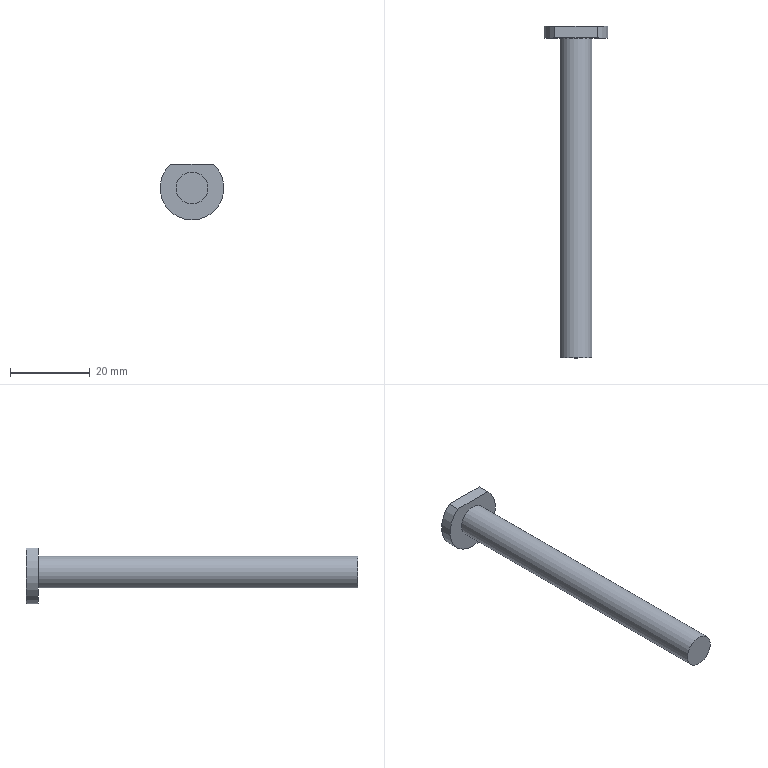Part | STEP file | latch post | 1 solid | 6 faces | box 16 x 83 x 14 mm | volume 4581 mm3 | plane 4 | cylinder 2 | commonest cylinder face diameters 8 x1 16 x1
STEP:
#1=CARTESIAN_POINT('',(0.,0.,0.));
#2=DIRECTION('',(0.,0.,1.));
#3=DIRECTION('',(1.,0.,0.));
#4=AXIS2_PLACEMENT_3D('',#1,#2,#3);
#5=CARTESIAN_POINT('',(-4.,80.,0.));
#6=VERTEX_POINT('',#5);
#7=CARTESIAN_POINT('',(0.,80.,0.));
#8=DIRECTION('',(0.,-1.,0.));
#9=DIRECTION('',(-1.,0.,0.));
#10=AXIS2_PLACEMENT_3D('',#7,#8,#9);
#11=CIRCLE('',#10,4.);
#12=CARTESIAN_POINT('',(0.,83.,0.));
#13=DIRECTION('',(0.,1.,0.));
#14=DIRECTION('',(-1.,0.,0.));
#15=AXIS2_PLACEMENT_3D('',#12,#13,#14);
#16=CYLINDRICAL_SURFACE('',#15,4.);
#17=CARTESIAN_POINT('',(6.283,-3.));
#18=DIRECTION('',(-1.,0.));
#19=VECTOR('',#18,1.);
#20=LINE('',#17,#19);
#21=(GEOMETRIC_REPRESENTATION_CONTEXT(2)PARAMETRIC_REPRESENTATION_CONTEXT()REPRESENTATION_CONTEXT('',''));
#22=DEFINITIONAL_REPRESENTATION('',(#20),#21);
#23=PCURVE('',#16,#22);
#24=CARTESIAN_POINT('',(4.,80.,0.));
#25=DIRECTION('',(0.,1.,0.));
#26=DIRECTION('',(-1.,0.,0.));
#27=AXIS2_PLACEMENT_3D('',#24,#25,#26);
#28=PLANE('',#27);
#29=CARTESIAN_POINT('',(8.,0.));
#30=CARTESIAN_POINT('',(8.,-6.928));
#31=CARTESIAN_POINT('',(2.,-3.464));
#32=CARTESIAN_POINT('',(-4.,0.));
#33=CARTESIAN_POINT('',(2.,3.464));
#34=CARTESIAN_POINT('',(8.,6.928));
#35=CARTESIAN_POINT('',(8.,0.));
#36=(BOUNDED_CURVE()B_SPLINE_CURVE(2,(#29,#30,#31,#32,#33,#34,#35),.UNSPECIFIED.,.T.,.F.)B_SPLINE_CURVE_WITH_KNOTS((1,2,2,2,2,1),(-2.094,0.,2.094,4.189,6.283,8.378),.UNSPECIFIED.)CURVE()GEOMETRIC_REPRESENTATION_ITEM()RATIONAL_B_SPLINE_CURVE((1.,0.5,1.,0.5,1.,0.5,1.))REPRESENTATION_ITEM(''));
#37=(GEOMETRIC_REPRESENTATION_CONTEXT(2)PARAMETRIC_REPRESENTATION_CONTEXT()REPRESENTATION_CONTEXT('',''));
#38=DEFINITIONAL_REPRESENTATION('',(#36),#37);
#39=PCURVE('',#28,#38);
#40=SURFACE_CURVE('',#11,(#23,#39),.PCURVE_S1.);
#41=EDGE_CURVE('',#6,#6,#40,.T.);
#42=ORIENTED_EDGE('',*,*,#41,.T.);
#43=CARTESIAN_POINT('',(-4.,0.,0.));
#44=VERTEX_POINT('',#43);
#45=CARTESIAN_POINT('',(-4.,0.,0.));
#46=CARTESIAN_POINT('',(-4.,80.,0.));
#47=B_SPLINE_CURVE_WITH_KNOTS('',1,(#45,#46),.UNSPECIFIED.,.F.,.F.,(2,2),(-83.,-3.),.PIECEWISE_BEZIER_KNOTS.);
#48=CARTESIAN_POINT('',(0.,0.));
#49=DIRECTION('',(0.,1.));
#50=VECTOR('',#49,1.);
#51=LINE('',#48,#50);
#52=(GEOMETRIC_REPRESENTATION_CONTEXT(2)PARAMETRIC_REPRESENTATION_CONTEXT()REPRESENTATION_CONTEXT('',''));
#53=DEFINITIONAL_REPRESENTATION('',(#51),#52);
#54=PCURVE('',#16,#53);
#55=CARTESIAN_POINT('',(6.283,0.));
#56=DIRECTION('',(0.,1.));
#57=VECTOR('',#56,1.);
#58=LINE('',#55,#57);
#59=(GEOMETRIC_REPRESENTATION_CONTEXT(2)PARAMETRIC_REPRESENTATION_CONTEXT()REPRESENTATION_CONTEXT('',''));
#60=DEFINITIONAL_REPRESENTATION('',(#58),#59);
#61=PCURVE('',#16,#60);
#62=SEAM_CURVE('',#47,(#54,#61),.PCURVE_S1.);
#63=EDGE_CURVE('',#44,#6,#62,.T.);
#64=ORIENTED_EDGE('',*,*,#63,.F.);
#65=CARTESIAN_POINT('',(0.,0.,0.));
#66=DIRECTION('',(0.,1.,0.));
#67=DIRECTION('',(-1.,0.,0.));
#68=AXIS2_PLACEMENT_3D('',#65,#66,#67);
#69=CIRCLE('',#68,4.);
#70=CARTESIAN_POINT('',(0.,-83.));
#71=DIRECTION('',(1.,0.));
#72=VECTOR('',#71,1.);
#73=LINE('',#70,#72);
#74=(GEOMETRIC_REPRESENTATION_CONTEXT(2)PARAMETRIC_REPRESENTATION_CONTEXT()REPRESENTATION_CONTEXT('',''));
#75=DEFINITIONAL_REPRESENTATION('',(#73),#74);
#76=PCURVE('',#16,#75);
#77=CARTESIAN_POINT('',(0.,0.,0.));
#78=DIRECTION('',(0.,1.,0.));
#79=DIRECTION('',(-1.,0.,0.));
#80=AXIS2_PLACEMENT_3D('',#77,#78,#79);
#81=PLANE('',#80);
#82=CARTESIAN_POINT('',(0.,0.));
#83=DIRECTION('',(1.,0.));
#84=AXIS2_PLACEMENT_2D('',#82,#83);
#85=CIRCLE('',#84,4.);
#86=(GEOMETRIC_REPRESENTATION_CONTEXT(2)PARAMETRIC_REPRESENTATION_CONTEXT()REPRESENTATION_CONTEXT('',''));
#87=DEFINITIONAL_REPRESENTATION('',(#85),#86);
#88=PCURVE('',#81,#87);
#89=SURFACE_CURVE('',#69,(#76,#88),.PCURVE_S1.);
#90=EDGE_CURVE('',#44,#44,#89,.T.);
#91=ORIENTED_EDGE('',*,*,#90,.T.);
#92=ORIENTED_EDGE('',*,*,#63,.T.);
#93=EDGE_LOOP('',(#42,#64,#91,#92));
#94=FACE_BOUND('',#93,.T.);
#95=ADVANCED_FACE('',(#94),#16,.T.);
#96=ORIENTED_EDGE('',*,*,#41,.F.);
#97=EDGE_LOOP('',(#96));
#98=FACE_BOUND('',#97,.T.);
#99=CARTESIAN_POINT('',(-5.292,80.,6.));
#100=VERTEX_POINT('',#99);
#101=CARTESIAN_POINT('',(5.292,80.,6.));
#102=VERTEX_POINT('',#101);
#103=CARTESIAN_POINT('',(4.,80.,6.));
#104=DIRECTION('',(1.,0.,0.));
#105=VECTOR('',#104,1.);
#106=LINE('',#103,#105);
#107=CARTESIAN_POINT('',(0.,6.));
#108=DIRECTION('',(-1.,0.));
#109=VECTOR('',#108,1.);
#110=LINE('',#107,#109);
#111=(GEOMETRIC_REPRESENTATION_CONTEXT(2)PARAMETRIC_REPRESENTATION_CONTEXT()REPRESENTATION_CONTEXT('',''));
#112=DEFINITIONAL_REPRESENTATION('',(#110),#111);
#113=PCURVE('',#28,#112);
#114=CARTESIAN_POINT('',(-5.292,73.,6.));
#115=DIRECTION('',(0.,0.,-1.));
#116=DIRECTION('',(-1.,0.,0.));
#117=AXIS2_PLACEMENT_3D('',#114,#115,#116);
#118=PLANE('',#117);
#119=CARTESIAN_POINT('',(-9.292,7.));
#120=DIRECTION('',(-1.,0.));
#121=VECTOR('',#120,1.);
#122=LINE('',#119,#121);
#123=(GEOMETRIC_REPRESENTATION_CONTEXT(2)PARAMETRIC_REPRESENTATION_CONTEXT()REPRESENTATION_CONTEXT('',''));
#124=DEFINITIONAL_REPRESENTATION('',(#122),#123);
#125=PCURVE('',#118,#124);
#126=SURFACE_CURVE('',#106,(#113,#125),.PCURVE_S1.);
#127=EDGE_CURVE('',#100,#102,#126,.T.);
#128=ORIENTED_EDGE('',*,*,#127,.F.);
#129=CARTESIAN_POINT('',(0.,80.,0.));
#130=DIRECTION('',(0.,1.,0.));
#131=DIRECTION('',(-1.,0.,0.));
#132=AXIS2_PLACEMENT_3D('',#129,#130,#131);
#133=CIRCLE('',#132,8.);
#134=CARTESIAN_POINT('',(4.,0.));
#135=DIRECTION('',(1.,0.));
#136=AXIS2_PLACEMENT_2D('',#134,#135);
#137=CIRCLE('',#136,8.);
#138=(GEOMETRIC_REPRESENTATION_CONTEXT(2)PARAMETRIC_REPRESENTATION_CONTEXT()REPRESENTATION_CONTEXT('',''));
#139=DEFINITIONAL_REPRESENTATION('',(#137),#138);
#140=PCURVE('',#28,#139);
#141=CARTESIAN_POINT('',(0.,83.,0.));
#142=DIRECTION('',(0.,1.,0.));
#143=DIRECTION('',(-1.,0.,0.));
#144=AXIS2_PLACEMENT_3D('',#141,#142,#143);
#145=CYLINDRICAL_SURFACE('',#144,8.);
#146=CARTESIAN_POINT('',(0.,-3.));
#147=DIRECTION('',(1.,0.));
#148=VECTOR('',#147,1.);
#149=LINE('',#146,#148);
#150=(GEOMETRIC_REPRESENTATION_CONTEXT(2)PARAMETRIC_REPRESENTATION_CONTEXT()REPRESENTATION_CONTEXT('',''));
#151=DEFINITIONAL_REPRESENTATION('',(#149),#150);
#152=PCURVE('',#145,#151);
#153=SURFACE_CURVE('',#133,(#140,#152),.PCURVE_S1.);
#154=EDGE_CURVE('',#102,#100,#153,.T.);
#155=ORIENTED_EDGE('',*,*,#154,.F.);
#156=EDGE_LOOP('',(#128,#155));
#157=FACE_BOUND('',#156,.T.);
#158=ADVANCED_FACE('',(#98,#157),#28,.F.);
#159=ORIENTED_EDGE('',*,*,#90,.F.);
#160=EDGE_LOOP('',(#159));
#161=FACE_BOUND('',#160,.T.);
#162=ADVANCED_FACE('',(#161),#81,.F.);
#163=CARTESIAN_POINT('',(-5.292,83.,6.));
#164=VERTEX_POINT('',#163);
#165=CARTESIAN_POINT('',(5.292,83.,6.));
#166=VERTEX_POINT('',#165);
#167=CARTESIAN_POINT('',(0.,83.,0.));
#168=DIRECTION('',(0.,-1.,0.));
#169=DIRECTION('',(-1.,0.,0.));
#170=AXIS2_PLACEMENT_3D('',#167,#168,#169);
#171=CIRCLE('',#170,8.);
#172=CARTESIAN_POINT('',(12.566,0.));
#173=DIRECTION('',(-1.,0.));
#174=VECTOR('',#173,1.);
#175=LINE('',#172,#174);
#176=(GEOMETRIC_REPRESENTATION_CONTEXT(2)PARAMETRIC_REPRESENTATION_CONTEXT()REPRESENTATION_CONTEXT('',''));
#177=DEFINITIONAL_REPRESENTATION('',(#175),#176);
#178=PCURVE('',#145,#177);
#179=CARTESIAN_POINT('',(8.,83.,0.));
#180=DIRECTION('',(0.,-1.,0.));
#181=DIRECTION('',(1.,0.,0.));
#182=AXIS2_PLACEMENT_3D('',#179,#180,#181);
#183=PLANE('',#182);
#184=CARTESIAN_POINT('',(-8.,0.));
#185=DIRECTION('',(-1.,0.));
#186=AXIS2_PLACEMENT_2D('',#184,#185);
#187=CIRCLE('',#186,8.);
#188=(GEOMETRIC_REPRESENTATION_CONTEXT(2)PARAMETRIC_REPRESENTATION_CONTEXT()REPRESENTATION_CONTEXT('',''));
#189=DEFINITIONAL_REPRESENTATION('',(#187),#188);
#190=PCURVE('',#183,#189);
#191=SURFACE_CURVE('',#171,(#178,#190),.PCURVE_S1.);
#192=EDGE_CURVE('',#164,#166,#191,.T.);
#193=ORIENTED_EDGE('',*,*,#192,.T.);
#194=CARTESIAN_POINT('',(5.292,83.,6.));
#195=DIRECTION('',(0.,-1.,0.));
#196=VECTOR('',#195,1.);
#197=LINE('',#194,#196);
#198=CARTESIAN_POINT('',(2.294,0.));
#199=DIRECTION('',(0.,-1.));
#200=VECTOR('',#199,1.);
#201=LINE('',#198,#200);
#202=(GEOMETRIC_REPRESENTATION_CONTEXT(2)PARAMETRIC_REPRESENTATION_CONTEXT()REPRESENTATION_CONTEXT('',''));
#203=DEFINITIONAL_REPRESENTATION('',(#201),#202);
#204=PCURVE('',#145,#203);
#205=CARTESIAN_POINT('',(-10.583,10.));
#206=DIRECTION('',(0.,-1.));
#207=VECTOR('',#206,1.);
#208=LINE('',#205,#207);
#209=(GEOMETRIC_REPRESENTATION_CONTEXT(2)PARAMETRIC_REPRESENTATION_CONTEXT()REPRESENTATION_CONTEXT('',''));
#210=DEFINITIONAL_REPRESENTATION('',(#208),#209);
#211=PCURVE('',#118,#210);
#212=SURFACE_CURVE('',#197,(#204,#211),.PCURVE_S1.);
#213=EDGE_CURVE('',#166,#102,#212,.T.);
#214=ORIENTED_EDGE('',*,*,#213,.T.);
#215=ORIENTED_EDGE('',*,*,#154,.T.);
#216=CARTESIAN_POINT('',(-5.292,73.,6.));
#217=DIRECTION('',(0.,1.,0.));
#218=VECTOR('',#217,1.);
#219=LINE('',#216,#218);
#220=CARTESIAN_POINT('',(7.131,-10.));
#221=DIRECTION('',(0.,1.));
#222=VECTOR('',#221,1.);
#223=LINE('',#220,#222);
#224=(GEOMETRIC_REPRESENTATION_CONTEXT(2)PARAMETRIC_REPRESENTATION_CONTEXT()REPRESENTATION_CONTEXT('',''));
#225=DEFINITIONAL_REPRESENTATION('',(#223),#224);
#226=PCURVE('',#145,#225);
#227=CARTESIAN_POINT('',(0.,0.));
#228=DIRECTION('',(0.,1.));
#229=VECTOR('',#228,1.);
#230=LINE('',#227,#229);
#231=(GEOMETRIC_REPRESENTATION_CONTEXT(2)PARAMETRIC_REPRESENTATION_CONTEXT()REPRESENTATION_CONTEXT('',''));
#232=DEFINITIONAL_REPRESENTATION('',(#230),#231);
#233=PCURVE('',#118,#232);
#234=SURFACE_CURVE('',#219,(#226,#233),.PCURVE_S1.);
#235=EDGE_CURVE('',#100,#164,#234,.T.);
#236=ORIENTED_EDGE('',*,*,#235,.T.);
#237=EDGE_LOOP('',(#193,#214,#215,#236));
#238=FACE_BOUND('',#237,.T.);
#239=ADVANCED_FACE('',(#238),#145,.T.);
#240=CARTESIAN_POINT('',(-5.292,83.,6.));
#241=DIRECTION('',(1.,0.,0.));
#242=VECTOR('',#241,1.);
#243=LINE('',#240,#242);
#244=CARTESIAN_POINT('',(0.,10.));
#245=DIRECTION('',(-1.,0.));
#246=VECTOR('',#245,1.);
#247=LINE('',#244,#246);
#248=(GEOMETRIC_REPRESENTATION_CONTEXT(2)PARAMETRIC_REPRESENTATION_CONTEXT()REPRESENTATION_CONTEXT('',''));
#249=DEFINITIONAL_REPRESENTATION('',(#247),#248);
#250=PCURVE('',#118,#249);
#251=CARTESIAN_POINT('',(-13.292,6.));
#252=DIRECTION('',(1.,0.));
#253=VECTOR('',#252,1.);
#254=LINE('',#251,#253);
#255=(GEOMETRIC_REPRESENTATION_CONTEXT(2)PARAMETRIC_REPRESENTATION_CONTEXT()REPRESENTATION_CONTEXT('',''));
#256=DEFINITIONAL_REPRESENTATION('',(#254),#255);
#257=PCURVE('',#183,#256);
#258=SURFACE_CURVE('',#243,(#250,#257),.PCURVE_S1.);
#259=EDGE_CURVE('',#164,#166,#258,.T.);
#260=ORIENTED_EDGE('',*,*,#259,.F.);
#261=ORIENTED_EDGE('',*,*,#235,.F.);
#262=ORIENTED_EDGE('',*,*,#127,.T.);
#263=ORIENTED_EDGE('',*,*,#213,.F.);
#264=EDGE_LOOP('',(#260,#261,#262,#263));
#265=FACE_BOUND('',#264,.T.);
#266=ADVANCED_FACE('',(#265),#118,.F.);
#267=ORIENTED_EDGE('',*,*,#192,.F.);
#268=ORIENTED_EDGE('',*,*,#259,.T.);
#269=EDGE_LOOP('',(#267,#268));
#270=FACE_BOUND('',#269,.T.);
#271=ADVANCED_FACE('',(#270),#183,.F.);
#272=CLOSED_SHELL('',(#95,#158,#162,#239,#266,#271));
#273=MANIFOLD_SOLID_BREP('',#272);
#274=(LENGTH_UNIT()NAMED_UNIT(*)SI_UNIT(.MILLI.,.METRE.));
#275=UNCERTAINTY_MEASURE_WITH_UNIT(LENGTH_MEASURE(0.000002),#274,'','');
#276=(NAMED_UNIT(*)PLANE_ANGLE_UNIT()SI_UNIT($,.RADIAN.));
#277=(NAMED_UNIT(*)SI_UNIT($,.STERADIAN.)SOLID_ANGLE_UNIT());
#278=(GEOMETRIC_REPRESENTATION_CONTEXT(3)GLOBAL_UNCERTAINTY_ASSIGNED_CONTEXT((#275))GLOBAL_UNIT_ASSIGNED_CONTEXT((#274,#276,#277))REPRESENTATION_CONTEXT('',''));
#279=ADVANCED_BREP_SHAPE_REPRESENTATION('',(#4,#273),#278);